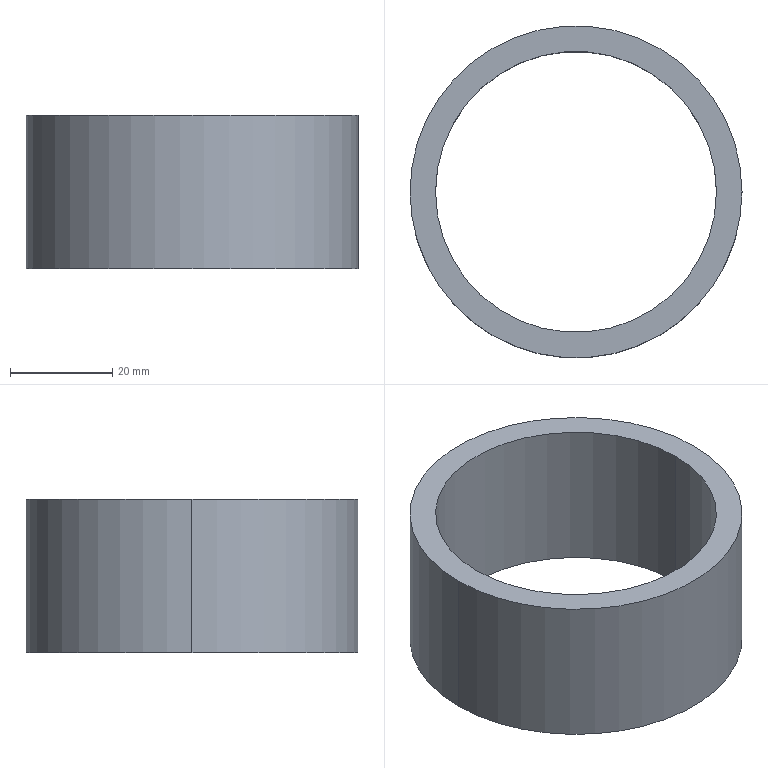Part | SolidWorks | features Extrusion 1 | 1 solid | 6 faces | box 65 x 65 x 30 mm | volume 28274 mm3 | cylinder 4 | plane 2 | commonest cylinder face diameters 55 x2 65 x2
STEP:
#1=CARTESIAN_POINT('',(-27.5,0.,30.));
#2=VERTEX_POINT('',#1);
#3=CARTESIAN_POINT('',(27.5,0.,30.));
#4=VERTEX_POINT('',#3);
#5=CARTESIAN_POINT('',(0.,0.,30.));
#6=DIRECTION('',(0.,0.,1.));
#7=DIRECTION('',(1.,0.,0.));
#8=AXIS2_PLACEMENT_3D('',#5,#6,#7);
#9=CIRCLE('',#8,27.5);
#10=EDGE_CURVE('',#2,#4,#9,.T.);
#11=ORIENTED_EDGE('',*,*,#10,.T.);
#12=CARTESIAN_POINT('',(27.5,0.,0.));
#13=VERTEX_POINT('',#12);
#14=CARTESIAN_POINT('',(27.5,0.,30.));
#15=DIRECTION('',(0.,0.,-1.));
#16=VECTOR('',#15,1000.);
#17=LINE('',#14,#16);
#18=EDGE_CURVE('',#4,#13,#17,.T.);
#19=ORIENTED_EDGE('',*,*,#18,.T.);
#20=CARTESIAN_POINT('',(-27.5,0.,0.));
#21=VERTEX_POINT('',#20);
#22=CARTESIAN_POINT('',(0.,0.,0.));
#23=DIRECTION('',(0.,0.,1.));
#24=DIRECTION('',(1.,0.,0.));
#25=AXIS2_PLACEMENT_3D('',#22,#23,#24);
#26=CIRCLE('',#25,27.5);
#27=EDGE_CURVE('',#21,#13,#26,.T.);
#28=ORIENTED_EDGE('',*,*,#27,.F.);
#29=CARTESIAN_POINT('',(-27.5,0.,30.));
#30=DIRECTION('',(0.,0.,-1.));
#31=VECTOR('',#30,1000.);
#32=LINE('',#29,#31);
#33=EDGE_CURVE('',#2,#21,#32,.T.);
#34=ORIENTED_EDGE('',*,*,#33,.F.);
#35=EDGE_LOOP('',(#11,#19,#28,#34));
#36=FACE_OUTER_BOUND('',#35,.T.);
#37=CARTESIAN_POINT('',(0.,0.,30.));
#38=DIRECTION('',(0.,0.,-1.));
#39=DIRECTION('',(-1.,0.,0.));
#40=AXIS2_PLACEMENT_3D('',#37,#38,#39);
#41=CYLINDRICAL_SURFACE('',#40,27.5);
#42=ADVANCED_FACE('',(#36),#41,.F.);
#43=CARTESIAN_POINT('',(32.5,0.,30.));
#44=VERTEX_POINT('',#43);
#45=CARTESIAN_POINT('',(-32.5,0.,30.));
#46=VERTEX_POINT('',#45);
#47=CARTESIAN_POINT('',(0.,0.,30.));
#48=DIRECTION('',(0.,0.,1.));
#49=DIRECTION('',(1.,0.,0.));
#50=AXIS2_PLACEMENT_3D('',#47,#48,#49);
#51=CIRCLE('',#50,32.5);
#52=EDGE_CURVE('',#44,#46,#51,.T.);
#53=ORIENTED_EDGE('',*,*,#52,.F.);
#54=CARTESIAN_POINT('',(32.5,0.,0.));
#55=VERTEX_POINT('',#54);
#56=CARTESIAN_POINT('',(32.5,0.,30.));
#57=DIRECTION('',(0.,0.,-1.));
#58=VECTOR('',#57,1000.);
#59=LINE('',#56,#58);
#60=EDGE_CURVE('',#44,#55,#59,.T.);
#61=ORIENTED_EDGE('',*,*,#60,.T.);
#62=CARTESIAN_POINT('',(-32.5,0.,0.));
#63=VERTEX_POINT('',#62);
#64=CARTESIAN_POINT('',(0.,0.,0.));
#65=DIRECTION('',(0.,0.,1.));
#66=DIRECTION('',(1.,0.,0.));
#67=AXIS2_PLACEMENT_3D('',#64,#65,#66);
#68=CIRCLE('',#67,32.5);
#69=EDGE_CURVE('',#55,#63,#68,.T.);
#70=ORIENTED_EDGE('',*,*,#69,.T.);
#71=CARTESIAN_POINT('',(-32.5,0.,30.));
#72=DIRECTION('',(0.,0.,-1.));
#73=VECTOR('',#72,1000.);
#74=LINE('',#71,#73);
#75=EDGE_CURVE('',#46,#63,#74,.T.);
#76=ORIENTED_EDGE('',*,*,#75,.F.);
#77=EDGE_LOOP('',(#53,#61,#70,#76));
#78=FACE_OUTER_BOUND('',#77,.T.);
#79=CARTESIAN_POINT('',(0.,0.,30.));
#80=DIRECTION('',(0.,0.,-1.));
#81=DIRECTION('',(-1.,0.,0.));
#82=AXIS2_PLACEMENT_3D('',#79,#80,#81);
#83=CYLINDRICAL_SURFACE('',#82,32.5);
#84=ADVANCED_FACE('',(#78),#83,.T.);
#85=CARTESIAN_POINT('',(0.,0.,30.));
#86=DIRECTION('',(0.,0.,1.));
#87=DIRECTION('',(1.,0.,0.));
#88=AXIS2_PLACEMENT_3D('',#85,#86,#87);
#89=CIRCLE('',#88,32.5);
#90=EDGE_CURVE('',#46,#44,#89,.T.);
#91=ORIENTED_EDGE('',*,*,#90,.T.);
#92=ORIENTED_EDGE('',*,*,#52,.T.);
#93=EDGE_LOOP('',(#91,#92));
#94=FACE_OUTER_BOUND('',#93,.T.);
#95=ORIENTED_EDGE('',*,*,#10,.F.);
#96=CARTESIAN_POINT('',(0.,0.,30.));
#97=DIRECTION('',(0.,0.,1.));
#98=DIRECTION('',(1.,0.,0.));
#99=AXIS2_PLACEMENT_3D('',#96,#97,#98);
#100=CIRCLE('',#99,27.5);
#101=EDGE_CURVE('',#4,#2,#100,.T.);
#102=ORIENTED_EDGE('',*,*,#101,.F.);
#103=EDGE_LOOP('',(#95,#102));
#104=FACE_BOUND('',#103,.T.);
#105=CARTESIAN_POINT('',(0.,0.,30.));
#106=DIRECTION('',(0.,0.,1.));
#107=DIRECTION('',(1.,0.,0.));
#108=AXIS2_PLACEMENT_3D('',#105,#106,#107);
#109=PLANE('',#108);
#110=ADVANCED_FACE('',(#94,#104),#109,.T.);
#111=CARTESIAN_POINT('',(0.,0.,0.));
#112=DIRECTION('',(0.,0.,1.));
#113=DIRECTION('',(1.,0.,0.));
#114=AXIS2_PLACEMENT_3D('',#111,#112,#113);
#115=CIRCLE('',#114,32.5);
#116=EDGE_CURVE('',#63,#55,#115,.T.);
#117=ORIENTED_EDGE('',*,*,#116,.F.);
#118=ORIENTED_EDGE('',*,*,#69,.F.);
#119=EDGE_LOOP('',(#117,#118));
#120=FACE_OUTER_BOUND('',#119,.T.);
#121=ORIENTED_EDGE('',*,*,#27,.T.);
#122=CARTESIAN_POINT('',(0.,0.,0.));
#123=DIRECTION('',(0.,0.,1.));
#124=DIRECTION('',(1.,0.,0.));
#125=AXIS2_PLACEMENT_3D('',#122,#123,#124);
#126=CIRCLE('',#125,27.5);
#127=EDGE_CURVE('',#13,#21,#126,.T.);
#128=ORIENTED_EDGE('',*,*,#127,.T.);
#129=EDGE_LOOP('',(#121,#128));
#130=FACE_BOUND('',#129,.T.);
#131=CARTESIAN_POINT('',(0.,0.,0.));
#132=DIRECTION('',(0.,0.,1.));
#133=DIRECTION('',(1.,0.,0.));
#134=AXIS2_PLACEMENT_3D('',#131,#132,#133);
#135=PLANE('',#134);
#136=ADVANCED_FACE('',(#120,#130),#135,.F.);
#137=ORIENTED_EDGE('',*,*,#60,.F.);
#138=ORIENTED_EDGE('',*,*,#90,.F.);
#139=ORIENTED_EDGE('',*,*,#75,.T.);
#140=ORIENTED_EDGE('',*,*,#116,.T.);
#141=EDGE_LOOP('',(#137,#138,#139,#140));
#142=FACE_OUTER_BOUND('',#141,.T.);
#143=CARTESIAN_POINT('',(0.,0.,30.));
#144=DIRECTION('',(0.,0.,-1.));
#145=DIRECTION('',(-1.,0.,0.));
#146=AXIS2_PLACEMENT_3D('',#143,#144,#145);
#147=CYLINDRICAL_SURFACE('',#146,32.5);
#148=ADVANCED_FACE('',(#142),#147,.T.);
#149=ORIENTED_EDGE('',*,*,#18,.F.);
#150=ORIENTED_EDGE('',*,*,#101,.T.);
#151=ORIENTED_EDGE('',*,*,#33,.T.);
#152=ORIENTED_EDGE('',*,*,#127,.F.);
#153=EDGE_LOOP('',(#149,#150,#151,#152));
#154=FACE_OUTER_BOUND('',#153,.T.);
#155=CARTESIAN_POINT('',(0.,0.,30.));
#156=DIRECTION('',(0.,0.,-1.));
#157=DIRECTION('',(-1.,0.,0.));
#158=AXIS2_PLACEMENT_3D('',#155,#156,#157);
#159=CYLINDRICAL_SURFACE('',#158,27.5);
#160=ADVANCED_FACE('',(#154),#159,.F.);
#161=CLOSED_SHELL('',(#42,#84,#110,#136,#148,#160));
#162=MANIFOLD_SOLID_BREP('',#161);
#163=CARTESIAN_POINT('',(0.,0.,0.));
#164=DIRECTION('',(0.,0.,1.));
#165=DIRECTION('',(1.,0.,0.));
#166=AXIS2_PLACEMENT_3D('',#163,#164,#165);
#167=(LENGTH_UNIT()NAMED_UNIT(*)SI_UNIT(.MILLI.,.METRE.));
#168=UNCERTAINTY_MEASURE_WITH_UNIT(LENGTH_MEASURE(0.00001),#167,'','');
#169=(NAMED_UNIT(*)PLANE_ANGLE_UNIT()SI_UNIT($,.RADIAN.));
#170=(NAMED_UNIT(*)SI_UNIT($,.STERADIAN.)SOLID_ANGLE_UNIT());
#171=(GEOMETRIC_REPRESENTATION_CONTEXT(3)GLOBAL_UNCERTAINTY_ASSIGNED_CONTEXT((#168))GLOBAL_UNIT_ASSIGNED_CONTEXT((#167,#169,#170))REPRESENTATION_CONTEXT('',''));
#172=ADVANCED_BREP_SHAPE_REPRESENTATION('',(#162,#166),#171);